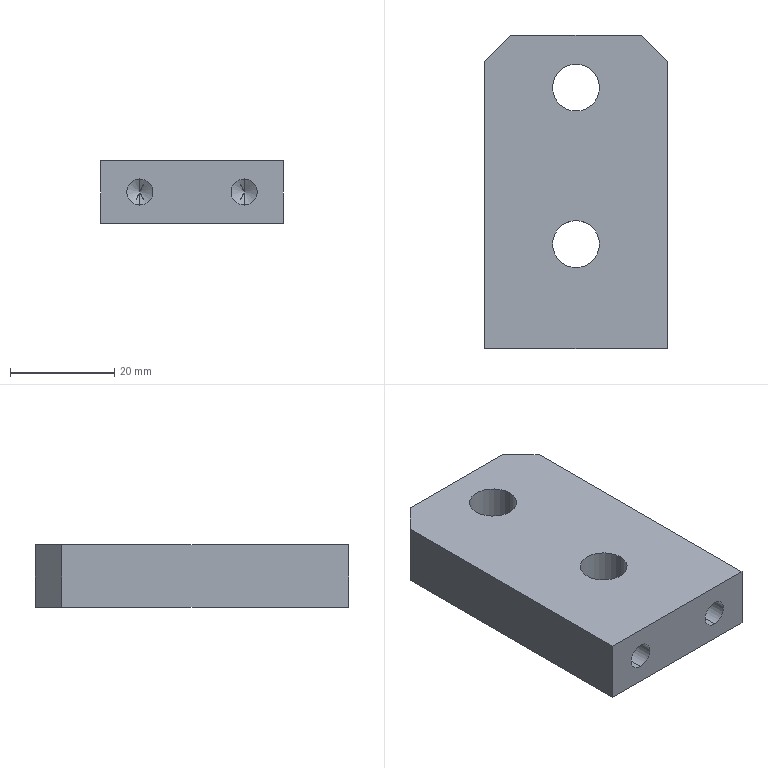Part | SolidWorks | features BaseBody 1 | 1 solid | 20 faces | box 35 x 60 x 12 mm | volume 22686 mm3 | cylinder 8 | plane 8 | cone 4 | commonest cylinder face diameters 5 x4 9 x4
STEP:
#1=CARTESIAN_POINT('',(-10.,-13.,8.5));
#2=VERTEX_POINT('',#1);
#3=CARTESIAN_POINT('',(-10.,-13.,3.5));
#4=VERTEX_POINT('',#3);
#5=CARTESIAN_POINT('',(-10.,-13.,6.));
#6=DIRECTION('',(0.,-1.,0.));
#7=DIRECTION('',(0.,0.,-1.));
#8=AXIS2_PLACEMENT_3D('',#5,#6,#7);
#9=CIRCLE('',#8,2.5);
#10=EDGE_CURVE('',#2,#4,#9,.T.);
#11=ORIENTED_EDGE('',*,*,#10,.F.);
#12=CARTESIAN_POINT('',(-10.,-30.,8.5));
#13=VERTEX_POINT('',#12);
#14=CARTESIAN_POINT('',(-10.,-30.,8.5));
#15=DIRECTION('',(0.,-1.,0.));
#16=VECTOR('',#15,1000.);
#17=LINE('',#14,#16);
#18=EDGE_CURVE('',#2,#13,#17,.T.);
#19=ORIENTED_EDGE('',*,*,#18,.T.);
#20=CARTESIAN_POINT('',(-10.,-30.,3.5));
#21=VERTEX_POINT('',#20);
#22=CARTESIAN_POINT('',(-10.,-30.,6.));
#23=DIRECTION('',(0.,-1.,0.));
#24=DIRECTION('',(0.,0.,-1.));
#25=AXIS2_PLACEMENT_3D('',#22,#23,#24);
#26=CIRCLE('',#25,2.5);
#27=EDGE_CURVE('',#13,#21,#26,.T.);
#28=ORIENTED_EDGE('',*,*,#27,.T.);
#29=CARTESIAN_POINT('',(-10.,-30.,3.5));
#30=DIRECTION('',(0.,-1.,0.));
#31=VECTOR('',#30,1000.);
#32=LINE('',#29,#31);
#33=EDGE_CURVE('',#4,#21,#32,.T.);
#34=ORIENTED_EDGE('',*,*,#33,.F.);
#35=EDGE_LOOP('',(#11,#19,#28,#34));
#36=FACE_OUTER_BOUND('',#35,.T.);
#37=CARTESIAN_POINT('',(-10.,-30.,6.));
#38=DIRECTION('',(0.,-1.,0.));
#39=DIRECTION('',(0.,0.,-1.));
#40=AXIS2_PLACEMENT_3D('',#37,#38,#39);
#41=CYLINDRICAL_SURFACE('',#40,2.5);
#42=ADVANCED_FACE('',(#36),#41,.F.);
#43=CARTESIAN_POINT('',(-10.,-11.498,6.));
#44=VERTEX_POINT('',#43);
#45=CARTESIAN_POINT('',(-10.,-13.,3.5));
#46=DIRECTION('',(0.,-0.515,-0.8572));
#47=VECTOR('',#46,1000.);
#48=LINE('',#45,#47);
#49=EDGE_CURVE('',#44,#4,#48,.T.);
#50=ORIENTED_EDGE('',*,*,#49,.F.);
#51=CARTESIAN_POINT('',(-10.,-13.,8.5));
#52=DIRECTION('',(0.,-0.515,0.8572));
#53=VECTOR('',#52,1000.);
#54=LINE('',#51,#53);
#55=EDGE_CURVE('',#44,#2,#54,.T.);
#56=ORIENTED_EDGE('',*,*,#55,.T.);
#57=ORIENTED_EDGE('',*,*,#10,.T.);
#58=EDGE_LOOP('',(#50,#56,#57));
#59=FACE_OUTER_BOUND('',#58,.T.);
#60=CARTESIAN_POINT('',(-10.,-13.,6.));
#61=DIRECTION('',(0.,-1.,0.));
#62=DIRECTION('',(0.,0.,-1.));
#63=AXIS2_PLACEMENT_3D('',#60,#61,#62);
#64=CONICAL_SURFACE('',#63,2.5,1.03);
#65=ADVANCED_FACE('',(#59),#64,.F.);
#66=CARTESIAN_POINT('',(10.,-13.,8.5));
#67=VERTEX_POINT('',#66);
#68=CARTESIAN_POINT('',(10.,-13.,3.5));
#69=VERTEX_POINT('',#68);
#70=CARTESIAN_POINT('',(10.,-13.,6.));
#71=DIRECTION('',(0.,-1.,0.));
#72=DIRECTION('',(0.,0.,-1.));
#73=AXIS2_PLACEMENT_3D('',#70,#71,#72);
#74=CIRCLE('',#73,2.5);
#75=EDGE_CURVE('',#67,#69,#74,.T.);
#76=ORIENTED_EDGE('',*,*,#75,.F.);
#77=CARTESIAN_POINT('',(10.,-30.,8.5));
#78=VERTEX_POINT('',#77);
#79=CARTESIAN_POINT('',(10.,-30.,8.5));
#80=DIRECTION('',(0.,-1.,0.));
#81=VECTOR('',#80,1000.);
#82=LINE('',#79,#81);
#83=EDGE_CURVE('',#67,#78,#82,.T.);
#84=ORIENTED_EDGE('',*,*,#83,.T.);
#85=CARTESIAN_POINT('',(10.,-30.,3.5));
#86=VERTEX_POINT('',#85);
#87=CARTESIAN_POINT('',(10.,-30.,6.));
#88=DIRECTION('',(0.,-1.,0.));
#89=DIRECTION('',(0.,0.,-1.));
#90=AXIS2_PLACEMENT_3D('',#87,#88,#89);
#91=CIRCLE('',#90,2.5);
#92=EDGE_CURVE('',#78,#86,#91,.T.);
#93=ORIENTED_EDGE('',*,*,#92,.T.);
#94=CARTESIAN_POINT('',(10.,-30.,3.5));
#95=DIRECTION('',(0.,-1.,0.));
#96=VECTOR('',#95,1000.);
#97=LINE('',#94,#96);
#98=EDGE_CURVE('',#69,#86,#97,.T.);
#99=ORIENTED_EDGE('',*,*,#98,.F.);
#100=EDGE_LOOP('',(#76,#84,#93,#99));
#101=FACE_OUTER_BOUND('',#100,.T.);
#102=CARTESIAN_POINT('',(10.,-30.,6.));
#103=DIRECTION('',(0.,-1.,0.));
#104=DIRECTION('',(0.,0.,-1.));
#105=AXIS2_PLACEMENT_3D('',#102,#103,#104);
#106=CYLINDRICAL_SURFACE('',#105,2.5);
#107=ADVANCED_FACE('',(#101),#106,.F.);
#108=CARTESIAN_POINT('',(10.,-11.498,6.));
#109=VERTEX_POINT('',#108);
#110=CARTESIAN_POINT('',(10.,-13.,3.5));
#111=DIRECTION('',(0.,-0.515,-0.8572));
#112=VECTOR('',#111,1000.);
#113=LINE('',#110,#112);
#114=EDGE_CURVE('',#109,#69,#113,.T.);
#115=ORIENTED_EDGE('',*,*,#114,.F.);
#116=CARTESIAN_POINT('',(10.,-13.,8.5));
#117=DIRECTION('',(0.,-0.515,0.8572));
#118=VECTOR('',#117,1000.);
#119=LINE('',#116,#118);
#120=EDGE_CURVE('',#109,#67,#119,.T.);
#121=ORIENTED_EDGE('',*,*,#120,.T.);
#122=ORIENTED_EDGE('',*,*,#75,.T.);
#123=EDGE_LOOP('',(#115,#121,#122));
#124=FACE_OUTER_BOUND('',#123,.T.);
#125=CARTESIAN_POINT('',(10.,-13.,6.));
#126=DIRECTION('',(0.,-1.,0.));
#127=DIRECTION('',(0.,0.,-1.));
#128=AXIS2_PLACEMENT_3D('',#125,#126,#127);
#129=CONICAL_SURFACE('',#128,2.5,1.03);
#130=ADVANCED_FACE('',(#124),#129,.F.);
#131=CARTESIAN_POINT('',(-4.5,20.,0.));
#132=VERTEX_POINT('',#131);
#133=CARTESIAN_POINT('',(4.5,20.,0.));
#134=VERTEX_POINT('',#133);
#135=CARTESIAN_POINT('',(0.,20.,0.));
#136=DIRECTION('',(0.,0.,1.));
#137=DIRECTION('',(1.,0.,0.));
#138=AXIS2_PLACEMENT_3D('',#135,#136,#137);
#139=CIRCLE('',#138,4.5);
#140=EDGE_CURVE('',#132,#134,#139,.T.);
#141=ORIENTED_EDGE('',*,*,#140,.F.);
#142=CARTESIAN_POINT('',(-4.5,20.,12.));
#143=VERTEX_POINT('',#142);
#144=CARTESIAN_POINT('',(-4.5,20.,12.));
#145=DIRECTION('',(0.,0.,1.));
#146=VECTOR('',#145,1000.);
#147=LINE('',#144,#146);
#148=EDGE_CURVE('',#132,#143,#147,.T.);
#149=ORIENTED_EDGE('',*,*,#148,.T.);
#150=CARTESIAN_POINT('',(4.5,20.,12.));
#151=VERTEX_POINT('',#150);
#152=CARTESIAN_POINT('',(0.,20.,12.));
#153=DIRECTION('',(0.,0.,1.));
#154=DIRECTION('',(1.,0.,0.));
#155=AXIS2_PLACEMENT_3D('',#152,#153,#154);
#156=CIRCLE('',#155,4.5);
#157=EDGE_CURVE('',#143,#151,#156,.T.);
#158=ORIENTED_EDGE('',*,*,#157,.T.);
#159=CARTESIAN_POINT('',(4.5,20.,12.));
#160=DIRECTION('',(0.,0.,1.));
#161=VECTOR('',#160,1000.);
#162=LINE('',#159,#161);
#163=EDGE_CURVE('',#134,#151,#162,.T.);
#164=ORIENTED_EDGE('',*,*,#163,.F.);
#165=EDGE_LOOP('',(#141,#149,#158,#164));
#166=FACE_OUTER_BOUND('',#165,.T.);
#167=CARTESIAN_POINT('',(0.,20.,12.));
#168=DIRECTION('',(0.,0.,1.));
#169=DIRECTION('',(1.,0.,0.));
#170=AXIS2_PLACEMENT_3D('',#167,#168,#169);
#171=CYLINDRICAL_SURFACE('',#170,4.5);
#172=ADVANCED_FACE('',(#166),#171,.F.);
#173=CARTESIAN_POINT('',(-4.5,-10.,0.));
#174=VERTEX_POINT('',#173);
#175=CARTESIAN_POINT('',(4.5,-10.,0.));
#176=VERTEX_POINT('',#175);
#177=CARTESIAN_POINT('',(0.,-10.,0.));
#178=DIRECTION('',(0.,0.,1.));
#179=DIRECTION('',(1.,0.,0.));
#180=AXIS2_PLACEMENT_3D('',#177,#178,#179);
#181=CIRCLE('',#180,4.5);
#182=EDGE_CURVE('',#174,#176,#181,.T.);
#183=ORIENTED_EDGE('',*,*,#182,.F.);
#184=CARTESIAN_POINT('',(-4.5,-10.,12.));
#185=VERTEX_POINT('',#184);
#186=CARTESIAN_POINT('',(-4.5,-10.,12.));
#187=DIRECTION('',(0.,0.,1.));
#188=VECTOR('',#187,1000.);
#189=LINE('',#186,#188);
#190=EDGE_CURVE('',#174,#185,#189,.T.);
#191=ORIENTED_EDGE('',*,*,#190,.T.);
#192=CARTESIAN_POINT('',(4.5,-10.,12.));
#193=VERTEX_POINT('',#192);
#194=CARTESIAN_POINT('',(0.,-10.,12.));
#195=DIRECTION('',(0.,0.,1.));
#196=DIRECTION('',(1.,0.,0.));
#197=AXIS2_PLACEMENT_3D('',#194,#195,#196);
#198=CIRCLE('',#197,4.5);
#199=EDGE_CURVE('',#185,#193,#198,.T.);
#200=ORIENTED_EDGE('',*,*,#199,.T.);
#201=CARTESIAN_POINT('',(4.5,-10.,12.));
#202=DIRECTION('',(0.,0.,1.));
#203=VECTOR('',#202,1000.);
#204=LINE('',#201,#203);
#205=EDGE_CURVE('',#176,#193,#204,.T.);
#206=ORIENTED_EDGE('',*,*,#205,.F.);
#207=EDGE_LOOP('',(#183,#191,#200,#206));
#208=FACE_OUTER_BOUND('',#207,.T.);
#209=CARTESIAN_POINT('',(0.,-10.,12.));
#210=DIRECTION('',(0.,0.,1.));
#211=DIRECTION('',(1.,0.,0.));
#212=AXIS2_PLACEMENT_3D('',#209,#210,#211);
#213=CYLINDRICAL_SURFACE('',#212,4.5);
#214=ADVANCED_FACE('',(#208),#213,.F.);
#215=CARTESIAN_POINT('',(17.5,-30.,0.));
#216=VERTEX_POINT('',#215);
#217=CARTESIAN_POINT('',(17.5,25.,0.));
#218=VERTEX_POINT('',#217);
#219=CARTESIAN_POINT('',(17.5,30.,0.));
#220=DIRECTION('',(0.,1.,0.));
#221=VECTOR('',#220,1000.);
#222=LINE('',#219,#221);
#223=EDGE_CURVE('',#216,#218,#222,.T.);
#224=ORIENTED_EDGE('',*,*,#223,.T.);
#225=CARTESIAN_POINT('',(17.5,25.,12.));
#226=VERTEX_POINT('',#225);
#227=CARTESIAN_POINT('',(17.5,25.,12.));
#228=DIRECTION('',(0.,0.,1.));
#229=VECTOR('',#228,1000.);
#230=LINE('',#227,#229);
#231=EDGE_CURVE('',#218,#226,#230,.T.);
#232=ORIENTED_EDGE('',*,*,#231,.T.);
#233=CARTESIAN_POINT('',(17.5,-30.,12.));
#234=VERTEX_POINT('',#233);
#235=CARTESIAN_POINT('',(17.5,30.,12.));
#236=DIRECTION('',(0.,1.,0.));
#237=VECTOR('',#236,1000.);
#238=LINE('',#235,#237);
#239=EDGE_CURVE('',#234,#226,#238,.T.);
#240=ORIENTED_EDGE('',*,*,#239,.F.);
#241=CARTESIAN_POINT('',(17.5,-30.,12.));
#242=DIRECTION('',(0.,0.,-1.));
#243=VECTOR('',#242,1000.);
#244=LINE('',#241,#243);
#245=EDGE_CURVE('',#234,#216,#244,.T.);
#246=ORIENTED_EDGE('',*,*,#245,.T.);
#247=EDGE_LOOP('',(#224,#232,#240,#246));
#248=FACE_OUTER_BOUND('',#247,.T.);
#249=CARTESIAN_POINT('',(17.5,30.,12.));
#250=DIRECTION('',(-1.,0.,0.));
#251=DIRECTION('',(0.,-1.,0.));
#252=AXIS2_PLACEMENT_3D('',#249,#250,#251);
#253=PLANE('',#252);
#254=ADVANCED_FACE('',(#248),#253,.F.);
#255=CARTESIAN_POINT('',(12.5,30.,0.));
#256=VERTEX_POINT('',#255);
#257=CARTESIAN_POINT('',(-12.5,30.,0.));
#258=VERTEX_POINT('',#257);
#259=CARTESIAN_POINT('',(-17.5,30.,0.));
#260=DIRECTION('',(-1.,0.,0.));
#261=VECTOR('',#260,1000.);
#262=LINE('',#259,#261);
#263=EDGE_CURVE('',#256,#258,#262,.T.);
#264=ORIENTED_EDGE('',*,*,#263,.T.);
#265=CARTESIAN_POINT('',(-12.5,30.,12.));
#266=VERTEX_POINT('',#265);
#267=CARTESIAN_POINT('',(-12.5,30.,12.));
#268=DIRECTION('',(0.,0.,1.));
#269=VECTOR('',#268,1000.);
#270=LINE('',#267,#269);
#271=EDGE_CURVE('',#258,#266,#270,.T.);
#272=ORIENTED_EDGE('',*,*,#271,.T.);
#273=CARTESIAN_POINT('',(12.5,30.,12.));
#274=VERTEX_POINT('',#273);
#275=CARTESIAN_POINT('',(-17.5,30.,12.));
#276=DIRECTION('',(-1.,0.,0.));
#277=VECTOR('',#276,1000.);
#278=LINE('',#275,#277);
#279=EDGE_CURVE('',#274,#266,#278,.T.);
#280=ORIENTED_EDGE('',*,*,#279,.F.);
#281=CARTESIAN_POINT('',(12.5,30.,12.));
#282=DIRECTION('',(0.,0.,-1.));
#283=VECTOR('',#282,1000.);
#284=LINE('',#281,#283);
#285=EDGE_CURVE('',#274,#256,#284,.T.);
#286=ORIENTED_EDGE('',*,*,#285,.T.);
#287=EDGE_LOOP('',(#264,#272,#280,#286));
#288=FACE_OUTER_BOUND('',#287,.T.);
#289=CARTESIAN_POINT('',(-17.5,30.,12.));
#290=DIRECTION('',(0.,-1.,0.));
#291=DIRECTION('',(0.,0.,-1.));
#292=AXIS2_PLACEMENT_3D('',#289,#290,#291);
#293=PLANE('',#292);
#294=ADVANCED_FACE('',(#288),#293,.F.);
#295=CARTESIAN_POINT('',(-17.5,25.,12.));
#296=VERTEX_POINT('',#295);
#297=CARTESIAN_POINT('',(-17.5,-30.,12.));
#298=VERTEX_POINT('',#297);
#299=CARTESIAN_POINT('',(-17.5,30.,12.));
#300=DIRECTION('',(0.,-1.,0.));
#301=VECTOR('',#300,1000.);
#302=LINE('',#299,#301);
#303=EDGE_CURVE('',#296,#298,#302,.T.);
#304=ORIENTED_EDGE('',*,*,#303,.F.);
#305=CARTESIAN_POINT('',(-17.5,25.,0.));
#306=VERTEX_POINT('',#305);
#307=CARTESIAN_POINT('',(-17.5,25.,12.));
#308=DIRECTION('',(0.,0.,-1.));
#309=VECTOR('',#308,1000.);
#310=LINE('',#307,#309);
#311=EDGE_CURVE('',#296,#306,#310,.T.);
#312=ORIENTED_EDGE('',*,*,#311,.T.);
#313=CARTESIAN_POINT('',(-17.5,-30.,0.));
#314=VERTEX_POINT('',#313);
#315=CARTESIAN_POINT('',(-17.5,30.,0.));
#316=DIRECTION('',(0.,-1.,0.));
#317=VECTOR('',#316,1000.);
#318=LINE('',#315,#317);
#319=EDGE_CURVE('',#306,#314,#318,.T.);
#320=ORIENTED_EDGE('',*,*,#319,.T.);
#321=CARTESIAN_POINT('',(-17.5,-30.,12.));
#322=DIRECTION('',(0.,0.,-1.));
#323=VECTOR('',#322,1000.);
#324=LINE('',#321,#323);
#325=EDGE_CURVE('',#298,#314,#324,.T.);
#326=ORIENTED_EDGE('',*,*,#325,.F.);
#327=EDGE_LOOP('',(#304,#312,#320,#326));
#328=FACE_OUTER_BOUND('',#327,.T.);
#329=CARTESIAN_POINT('',(-17.5,30.,12.));
#330=DIRECTION('',(1.,0.,0.));
#331=DIRECTION('',(0.,1.,0.));
#332=AXIS2_PLACEMENT_3D('',#329,#330,#331);
#333=PLANE('',#332);
#334=ADVANCED_FACE('',(#328),#333,.F.);
#335=CARTESIAN_POINT('',(-10.,-30.,6.));
#336=DIRECTION('',(0.,-1.,0.));
#337=DIRECTION('',(0.,0.,-1.));
#338=AXIS2_PLACEMENT_3D('',#335,#336,#337);
#339=CIRCLE('',#338,2.5);
#340=EDGE_CURVE('',#21,#13,#339,.T.);
#341=ORIENTED_EDGE('',*,*,#340,.F.);
#342=ORIENTED_EDGE('',*,*,#27,.F.);
#343=EDGE_LOOP('',(#341,#342));
#344=FACE_BOUND('',#343,.T.);
#345=CARTESIAN_POINT('',(10.,-30.,6.));
#346=DIRECTION('',(0.,-1.,0.));
#347=DIRECTION('',(0.,0.,-1.));
#348=AXIS2_PLACEMENT_3D('',#345,#346,#347);
#349=CIRCLE('',#348,2.5);
#350=EDGE_CURVE('',#86,#78,#349,.T.);
#351=ORIENTED_EDGE('',*,*,#350,.F.);
#352=ORIENTED_EDGE('',*,*,#92,.F.);
#353=EDGE_LOOP('',(#351,#352));
#354=FACE_BOUND('',#353,.T.);
#355=CARTESIAN_POINT('',(-17.5,-30.,0.));
#356=DIRECTION('',(1.,0.,0.));
#357=VECTOR('',#356,1000.);
#358=LINE('',#355,#357);
#359=EDGE_CURVE('',#314,#216,#358,.T.);
#360=ORIENTED_EDGE('',*,*,#359,.T.);
#361=ORIENTED_EDGE('',*,*,#245,.F.);
#362=CARTESIAN_POINT('',(-17.5,-30.,12.));
#363=DIRECTION('',(1.,0.,0.));
#364=VECTOR('',#363,1000.);
#365=LINE('',#362,#364);
#366=EDGE_CURVE('',#298,#234,#365,.T.);
#367=ORIENTED_EDGE('',*,*,#366,.F.);
#368=ORIENTED_EDGE('',*,*,#325,.T.);
#369=EDGE_LOOP('',(#360,#361,#367,#368));
#370=FACE_OUTER_BOUND('',#369,.T.);
#371=CARTESIAN_POINT('',(-17.5,-30.,12.));
#372=DIRECTION('',(0.,1.,0.));
#373=DIRECTION('',(0.,0.,1.));
#374=AXIS2_PLACEMENT_3D('',#371,#372,#373);
#375=PLANE('',#374);
#376=ADVANCED_FACE('',(#344,#354,#370),#375,.F.);
#377=CARTESIAN_POINT('',(0.,20.,12.));
#378=DIRECTION('',(0.,0.,1.));
#379=DIRECTION('',(1.,0.,0.));
#380=AXIS2_PLACEMENT_3D('',#377,#378,#379);
#381=CIRCLE('',#380,4.5);
#382=EDGE_CURVE('',#151,#143,#381,.T.);
#383=ORIENTED_EDGE('',*,*,#382,.F.);
#384=ORIENTED_EDGE('',*,*,#157,.F.);
#385=EDGE_LOOP('',(#383,#384));
#386=FACE_BOUND('',#385,.T.);
#387=CARTESIAN_POINT('',(0.,-10.,12.));
#388=DIRECTION('',(0.,0.,1.));
#389=DIRECTION('',(1.,0.,0.));
#390=AXIS2_PLACEMENT_3D('',#387,#388,#389);
#391=CIRCLE('',#390,4.5);
#392=EDGE_CURVE('',#193,#185,#391,.T.);
#393=ORIENTED_EDGE('',*,*,#392,.F.);
#394=ORIENTED_EDGE('',*,*,#199,.F.);
#395=EDGE_LOOP('',(#393,#394));
#396=FACE_BOUND('',#395,.T.);
#397=ORIENTED_EDGE('',*,*,#279,.T.);
#398=CARTESIAN_POINT('',(-21.25,21.25,12.));
#399=DIRECTION('',(-0.7071,-0.7071,0.));
#400=VECTOR('',#399,1000.);
#401=LINE('',#398,#400);
#402=EDGE_CURVE('',#266,#296,#401,.T.);
#403=ORIENTED_EDGE('',*,*,#402,.T.);
#404=ORIENTED_EDGE('',*,*,#303,.T.);
#405=ORIENTED_EDGE('',*,*,#366,.T.);
#406=ORIENTED_EDGE('',*,*,#239,.T.);
#407=CARTESIAN_POINT('',(21.25,21.25,12.));
#408=DIRECTION('',(-0.7071,0.7071,0.));
#409=VECTOR('',#408,1000.);
#410=LINE('',#407,#409);
#411=EDGE_CURVE('',#226,#274,#410,.T.);
#412=ORIENTED_EDGE('',*,*,#411,.T.);
#413=EDGE_LOOP('',(#397,#403,#404,#405,#406,#412));
#414=FACE_OUTER_BOUND('',#413,.T.);
#415=CARTESIAN_POINT('',(0.,0.,12.));
#416=DIRECTION('',(0.,0.,1.));
#417=DIRECTION('',(1.,0.,0.));
#418=AXIS2_PLACEMENT_3D('',#415,#416,#417);
#419=PLANE('',#418);
#420=ADVANCED_FACE('',(#386,#396,#414),#419,.T.);
#421=CARTESIAN_POINT('',(0.,20.,0.));
#422=DIRECTION('',(0.,0.,1.));
#423=DIRECTION('',(1.,0.,0.));
#424=AXIS2_PLACEMENT_3D('',#421,#422,#423);
#425=CIRCLE('',#424,4.5);
#426=EDGE_CURVE('',#134,#132,#425,.T.);
#427=ORIENTED_EDGE('',*,*,#426,.T.);
#428=ORIENTED_EDGE('',*,*,#140,.T.);
#429=EDGE_LOOP('',(#427,#428));
#430=FACE_BOUND('',#429,.T.);
#431=CARTESIAN_POINT('',(0.,-10.,0.));
#432=DIRECTION('',(0.,0.,1.));
#433=DIRECTION('',(1.,0.,0.));
#434=AXIS2_PLACEMENT_3D('',#431,#432,#433);
#435=CIRCLE('',#434,4.5);
#436=EDGE_CURVE('',#176,#174,#435,.T.);
#437=ORIENTED_EDGE('',*,*,#436,.T.);
#438=ORIENTED_EDGE('',*,*,#182,.T.);
#439=EDGE_LOOP('',(#437,#438));
#440=FACE_BOUND('',#439,.T.);
#441=ORIENTED_EDGE('',*,*,#319,.F.);
#442=CARTESIAN_POINT('',(-17.5,25.,0.));
#443=DIRECTION('',(0.7071,0.7071,0.));
#444=VECTOR('',#443,1000.);
#445=LINE('',#442,#444);
#446=EDGE_CURVE('',#306,#258,#445,.T.);
#447=ORIENTED_EDGE('',*,*,#446,.T.);
#448=ORIENTED_EDGE('',*,*,#263,.F.);
#449=CARTESIAN_POINT('',(12.5,30.,0.));
#450=DIRECTION('',(0.7071,-0.7071,0.));
#451=VECTOR('',#450,1000.);
#452=LINE('',#449,#451);
#453=EDGE_CURVE('',#256,#218,#452,.T.);
#454=ORIENTED_EDGE('',*,*,#453,.T.);
#455=ORIENTED_EDGE('',*,*,#223,.F.);
#456=ORIENTED_EDGE('',*,*,#359,.F.);
#457=EDGE_LOOP('',(#441,#447,#448,#454,#455,#456));
#458=FACE_OUTER_BOUND('',#457,.T.);
#459=CARTESIAN_POINT('',(0.,0.,0.));
#460=DIRECTION('',(0.,0.,1.));
#461=DIRECTION('',(1.,0.,0.));
#462=AXIS2_PLACEMENT_3D('',#459,#460,#461);
#463=PLANE('',#462);
#464=ADVANCED_FACE('',(#430,#440,#458),#463,.F.);
#465=ORIENTED_EDGE('',*,*,#402,.F.);
#466=ORIENTED_EDGE('',*,*,#271,.F.);
#467=ORIENTED_EDGE('',*,*,#446,.F.);
#468=ORIENTED_EDGE('',*,*,#311,.F.);
#469=EDGE_LOOP('',(#465,#466,#467,#468));
#470=FACE_OUTER_BOUND('',#469,.T.);
#471=CARTESIAN_POINT('',(-17.5,25.,12.));
#472=DIRECTION('',(0.7071,-0.7071,0.));
#473=DIRECTION('',(0.,0.,-1.));
#474=AXIS2_PLACEMENT_3D('',#471,#472,#473);
#475=PLANE('',#474);
#476=ADVANCED_FACE('',(#470),#475,.F.);
#477=ORIENTED_EDGE('',*,*,#411,.F.);
#478=ORIENTED_EDGE('',*,*,#231,.F.);
#479=ORIENTED_EDGE('',*,*,#453,.F.);
#480=ORIENTED_EDGE('',*,*,#285,.F.);
#481=EDGE_LOOP('',(#477,#478,#479,#480));
#482=FACE_OUTER_BOUND('',#481,.T.);
#483=CARTESIAN_POINT('',(12.5,30.,12.));
#484=DIRECTION('',(-0.7071,-0.7071,0.));
#485=DIRECTION('',(0.,0.,-1.));
#486=AXIS2_PLACEMENT_3D('',#483,#484,#485);
#487=PLANE('',#486);
#488=ADVANCED_FACE('',(#482),#487,.F.);
#489=ORIENTED_EDGE('',*,*,#190,.F.);
#490=ORIENTED_EDGE('',*,*,#436,.F.);
#491=ORIENTED_EDGE('',*,*,#205,.T.);
#492=ORIENTED_EDGE('',*,*,#392,.T.);
#493=EDGE_LOOP('',(#489,#490,#491,#492));
#494=FACE_OUTER_BOUND('',#493,.T.);
#495=CARTESIAN_POINT('',(0.,-10.,12.));
#496=DIRECTION('',(0.,0.,1.));
#497=DIRECTION('',(1.,0.,0.));
#498=AXIS2_PLACEMENT_3D('',#495,#496,#497);
#499=CYLINDRICAL_SURFACE('',#498,4.5);
#500=ADVANCED_FACE('',(#494),#499,.F.);
#501=ORIENTED_EDGE('',*,*,#148,.F.);
#502=ORIENTED_EDGE('',*,*,#426,.F.);
#503=ORIENTED_EDGE('',*,*,#163,.T.);
#504=ORIENTED_EDGE('',*,*,#382,.T.);
#505=EDGE_LOOP('',(#501,#502,#503,#504));
#506=FACE_OUTER_BOUND('',#505,.T.);
#507=CARTESIAN_POINT('',(0.,20.,12.));
#508=DIRECTION('',(0.,0.,1.));
#509=DIRECTION('',(1.,0.,0.));
#510=AXIS2_PLACEMENT_3D('',#507,#508,#509);
#511=CYLINDRICAL_SURFACE('',#510,4.5);
#512=ADVANCED_FACE('',(#506),#511,.F.);
#513=ORIENTED_EDGE('',*,*,#120,.F.);
#514=ORIENTED_EDGE('',*,*,#114,.T.);
#515=CARTESIAN_POINT('',(10.,-13.,6.));
#516=DIRECTION('',(0.,-1.,0.));
#517=DIRECTION('',(0.,0.,-1.));
#518=AXIS2_PLACEMENT_3D('',#515,#516,#517);
#519=CIRCLE('',#518,2.5);
#520=EDGE_CURVE('',#69,#67,#519,.T.);
#521=ORIENTED_EDGE('',*,*,#520,.T.);
#522=EDGE_LOOP('',(#513,#514,#521));
#523=FACE_OUTER_BOUND('',#522,.T.);
#524=CARTESIAN_POINT('',(10.,-13.,6.));
#525=DIRECTION('',(0.,-1.,0.));
#526=DIRECTION('',(0.,0.,-1.));
#527=AXIS2_PLACEMENT_3D('',#524,#525,#526);
#528=CONICAL_SURFACE('',#527,2.5,1.03);
#529=ADVANCED_FACE('',(#523),#528,.F.);
#530=ORIENTED_EDGE('',*,*,#83,.F.);
#531=ORIENTED_EDGE('',*,*,#520,.F.);
#532=ORIENTED_EDGE('',*,*,#98,.T.);
#533=ORIENTED_EDGE('',*,*,#350,.T.);
#534=EDGE_LOOP('',(#530,#531,#532,#533));
#535=FACE_OUTER_BOUND('',#534,.T.);
#536=CARTESIAN_POINT('',(10.,-30.,6.));
#537=DIRECTION('',(0.,-1.,0.));
#538=DIRECTION('',(0.,0.,-1.));
#539=AXIS2_PLACEMENT_3D('',#536,#537,#538);
#540=CYLINDRICAL_SURFACE('',#539,2.5);
#541=ADVANCED_FACE('',(#535),#540,.F.);
#542=ORIENTED_EDGE('',*,*,#55,.F.);
#543=ORIENTED_EDGE('',*,*,#49,.T.);
#544=CARTESIAN_POINT('',(-10.,-13.,6.));
#545=DIRECTION('',(0.,-1.,0.));
#546=DIRECTION('',(0.,0.,-1.));
#547=AXIS2_PLACEMENT_3D('',#544,#545,#546);
#548=CIRCLE('',#547,2.5);
#549=EDGE_CURVE('',#4,#2,#548,.T.);
#550=ORIENTED_EDGE('',*,*,#549,.T.);
#551=EDGE_LOOP('',(#542,#543,#550));
#552=FACE_OUTER_BOUND('',#551,.T.);
#553=CARTESIAN_POINT('',(-10.,-13.,6.));
#554=DIRECTION('',(0.,-1.,0.));
#555=DIRECTION('',(0.,0.,-1.));
#556=AXIS2_PLACEMENT_3D('',#553,#554,#555);
#557=CONICAL_SURFACE('',#556,2.5,1.03);
#558=ADVANCED_FACE('',(#552),#557,.F.);
#559=ORIENTED_EDGE('',*,*,#18,.F.);
#560=ORIENTED_EDGE('',*,*,#549,.F.);
#561=ORIENTED_EDGE('',*,*,#33,.T.);
#562=ORIENTED_EDGE('',*,*,#340,.T.);
#563=EDGE_LOOP('',(#559,#560,#561,#562));
#564=FACE_OUTER_BOUND('',#563,.T.);
#565=CARTESIAN_POINT('',(-10.,-30.,6.));
#566=DIRECTION('',(0.,-1.,0.));
#567=DIRECTION('',(0.,0.,-1.));
#568=AXIS2_PLACEMENT_3D('',#565,#566,#567);
#569=CYLINDRICAL_SURFACE('',#568,2.5);
#570=ADVANCED_FACE('',(#564),#569,.F.);
#571=CLOSED_SHELL('',(#42,#65,#107,#130,#172,#214,#254,#294,#334,#376,#420,#464,#476,#488,#500,#512,#529,#541,#558,#570));
#572=MANIFOLD_SOLID_BREP('',#571);
#573=CARTESIAN_POINT('',(0.,0.,0.));
#574=DIRECTION('',(0.,0.,1.));
#575=DIRECTION('',(1.,0.,0.));
#576=AXIS2_PLACEMENT_3D('',#573,#574,#575);
#577=(LENGTH_UNIT()NAMED_UNIT(*)SI_UNIT(.MILLI.,.METRE.));
#578=UNCERTAINTY_MEASURE_WITH_UNIT(LENGTH_MEASURE(0.00001),#577,'','');
#579=(NAMED_UNIT(*)PLANE_ANGLE_UNIT()SI_UNIT($,.RADIAN.));
#580=(NAMED_UNIT(*)SI_UNIT($,.STERADIAN.)SOLID_ANGLE_UNIT());
#581=(GEOMETRIC_REPRESENTATION_CONTEXT(3)GLOBAL_UNCERTAINTY_ASSIGNED_CONTEXT((#578))GLOBAL_UNIT_ASSIGNED_CONTEXT((#577,#579,#580))REPRESENTATION_CONTEXT('',''));
#582=ADVANCED_BREP_SHAPE_REPRESENTATION('',(#572,#576),#581);